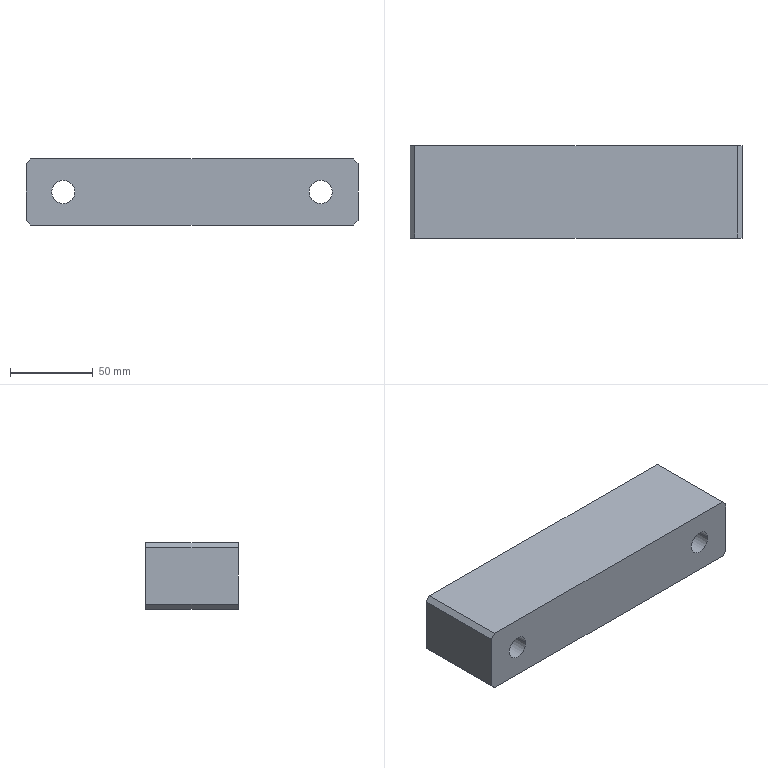Part | STEP file | J452-EBZ05-04-04-Part-1 | 1 solid | 34 faces | box 200 x 55.5 x 40 mm | volume 402203 mm3 | cylinder 16 | plane 14 | cone 4 | commonest cylinder face diameters 14 x8 16 x4 20 x4